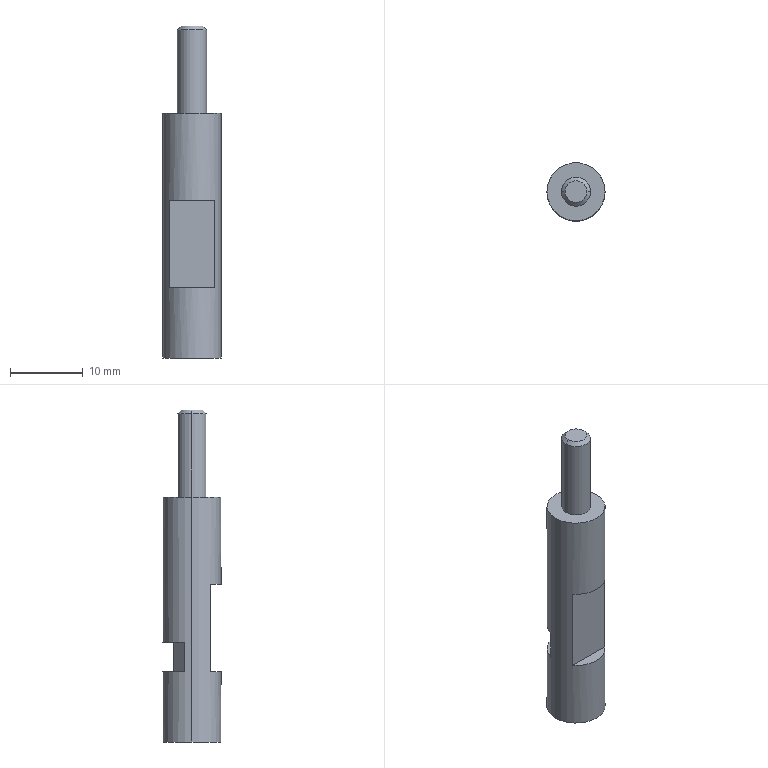Part | SolidWorks | features ICE 4, 3DProfileFeature 2, HoleWzd 2, Chamfer 1, Extrusion 1, RefAxis 1 | 1 solid | 24 faces | box 8 x 8 x 45.7 mm | volume 1609 mm3 | plane 11 | cylinder 8 | cone 5 | commonest cylinder face diameters 3.2 x4 4 x2 8 x2
STEP:
#1=CARTESIAN_POINT('',(-0.02022,1.6,10.1));
#2=VERTEX_POINT('',#1);
#3=CARTESIAN_POINT('',(-1.6,0.,11.446));
#4=VERTEX_POINT('',#3);
#5=CARTESIAN_POINT('',(-0.02022,1.6,10.1));
#6=CARTESIAN_POINT('',(-0.1403,1.598,10.1));
#7=CARTESIAN_POINT('',(-0.2616,1.583,10.114));
#8=CARTESIAN_POINT('',(-0.4907,1.527,10.166));
#9=CARTESIAN_POINT('',(-0.6,1.487,10.205));
#10=CARTESIAN_POINT('',(-0.8999,1.342,10.345));
#11=CARTESIAN_POINT('',(-1.065,1.21,10.473));
#12=CARTESIAN_POINT('',(-1.324,0.9196,10.753));
#13=CARTESIAN_POINT('',(-1.421,0.7579,10.908));
#14=CARTESIAN_POINT('',(-1.522,0.5024,11.141));
#15=CARTESIAN_POINT('',(-1.548,0.4151,11.219));
#16=CARTESIAN_POINT('',(-1.577,0.274,11.329));
#17=CARTESIAN_POINT('',(-1.585,0.225,11.365));
#18=CARTESIAN_POINT('',(-1.596,0.1195,11.423));
#19=CARTESIAN_POINT('',(-1.6,0.06134,11.446));
#20=CARTESIAN_POINT('',(-1.6,0.,11.446));
#21=B_SPLINE_CURVE_WITH_KNOTS('',3,(#5,#6,#7,#8,#9,#10,#11,#12,#13,#14,#15,#16,#17,#18,#19,#20),.UNSPECIFIED.,.F.,.F.,(4,2,2,2,2,2,2,4),(0.008715,0.009076,0.009436,0.01016,0.01088,0.01124,0.01142,0.0116),.UNSPECIFIED.);
#22=EDGE_CURVE('',#2,#4,#21,.T.);
#23=ORIENTED_EDGE('',*,*,#22,.F.);
#24=CARTESIAN_POINT('',(-0.02022,2.5,10.1));
#25=VERTEX_POINT('',#24);
#26=CARTESIAN_POINT('',(-0.02022,2.5,10.1));
#27=DIRECTION('',(0.,1.,0.));
#28=VECTOR('',#27,1000.);
#29=LINE('',#26,#28);
#30=EDGE_CURVE('',#2,#25,#29,.T.);
#31=ORIENTED_EDGE('',*,*,#30,.T.);
#32=CARTESIAN_POINT('',(-0.02022,2.5,13.3));
#33=VERTEX_POINT('',#32);
#34=CARTESIAN_POINT('',(-0.02022,2.5,11.7));
#35=DIRECTION('',(0.,1.,0.));
#36=DIRECTION('',(0.,0.,1.));
#37=AXIS2_PLACEMENT_3D('',#34,#35,#36);
#38=CIRCLE('',#37,1.6);
#39=EDGE_CURVE('',#25,#33,#38,.T.);
#40=ORIENTED_EDGE('',*,*,#39,.T.);
#41=CARTESIAN_POINT('',(-0.02022,1.6,13.3));
#42=VERTEX_POINT('',#41);
#43=CARTESIAN_POINT('',(-0.02022,2.5,13.3));
#44=DIRECTION('',(0.,1.,0.));
#45=VECTOR('',#44,1000.);
#46=LINE('',#43,#45);
#47=EDGE_CURVE('',#42,#33,#46,.T.);
#48=ORIENTED_EDGE('',*,*,#47,.F.);
#49=CARTESIAN_POINT('',(-1.6,0.,11.954));
#50=VERTEX_POINT('',#49);
#51=CARTESIAN_POINT('',(-1.6,0.,11.954));
#52=CARTESIAN_POINT('',(-1.6,0.06178,11.954));
#53=CARTESIAN_POINT('',(-1.596,0.1196,11.977));
#54=CARTESIAN_POINT('',(-1.585,0.2248,12.035));
#55=CARTESIAN_POINT('',(-1.577,0.2732,12.07));
#56=CARTESIAN_POINT('',(-1.548,0.4148,12.18));
#57=CARTESIAN_POINT('',(-1.522,0.5025,12.259));
#58=CARTESIAN_POINT('',(-1.455,0.6723,12.414));
#59=CARTESIAN_POINT('',(-1.414,0.7543,12.491));
#60=CARTESIAN_POINT('',(-1.317,0.9136,12.642));
#61=CARTESIAN_POINT('',(-1.26,0.9914,12.716));
#62=CARTESIAN_POINT('',(-1.13,1.137,12.857));
#63=CARTESIAN_POINT('',(-1.057,1.206,12.923));
#64=CARTESIAN_POINT('',(-0.8918,1.332,13.046));
#65=CARTESIAN_POINT('',(-0.7997,1.39,13.102));
#66=CARTESIAN_POINT('',(-0.6006,1.487,13.195));
#67=CARTESIAN_POINT('',(-0.4907,1.527,13.234));
#68=CARTESIAN_POINT('',(-0.2622,1.583,13.286));
#69=CARTESIAN_POINT('',(-0.1408,1.598,13.3));
#70=CARTESIAN_POINT('',(-0.02022,1.6,13.3));
#71=B_SPLINE_CURVE_WITH_KNOTS('',3,(#51,#52,#53,#54,#55,#56,#57,#58,#59,#60,#61,#62,#63,#64,#65,#66,#67,#68,#69,#70),.UNSPECIFIED.,.F.,.F.,(4,2,2,2,2,2,2,2,2,4),(0.,0.000181,0.000362,0.0007239,0.001086,0.001448,0.00181,0.002172,0.002534,0.002896),.UNSPECIFIED.);
#72=EDGE_CURVE('',#50,#42,#71,.T.);
#73=ORIENTED_EDGE('',*,*,#72,.F.);
#74=CARTESIAN_POINT('',(-0.02022,0.,11.7));
#75=DIRECTION('',(0.,1.,0.));
#76=DIRECTION('',(0.,0.,1.));
#77=AXIS2_PLACEMENT_3D('',#74,#75,#76);
#78=CIRCLE('',#77,1.6);
#79=EDGE_CURVE('',#4,#50,#78,.T.);
#80=ORIENTED_EDGE('',*,*,#79,.F.);
#81=EDGE_LOOP('',(#23,#31,#40,#48,#73,#80));
#82=FACE_OUTER_BOUND('',#81,.T.);
#83=CARTESIAN_POINT('',(-0.02022,2.5,11.7));
#84=DIRECTION('',(0.,1.,0.));
#85=DIRECTION('',(0.,0.,1.));
#86=AXIS2_PLACEMENT_3D('',#83,#84,#85);
#87=CYLINDRICAL_SURFACE('',#86,1.6);
#88=ADVANCED_FACE('',(#82),#87,.F.);
#89=CARTESIAN_POINT('',(1.6,0.,14.));
#90=VERTEX_POINT('',#89);
#91=CARTESIAN_POINT('',(-1.6,0.,14.));
#92=VERTEX_POINT('',#91);
#93=CARTESIAN_POINT('',(0.,0.,14.));
#94=DIRECTION('',(0.,0.,-1.));
#95=DIRECTION('',(-1.,0.,0.));
#96=AXIS2_PLACEMENT_3D('',#93,#94,#95);
#97=CIRCLE('',#96,1.6);
#98=EDGE_CURVE('',#90,#92,#97,.T.);
#99=ORIENTED_EDGE('',*,*,#98,.F.);
#100=CARTESIAN_POINT('',(1.6,0.,0.));
#101=VERTEX_POINT('',#100);
#102=CARTESIAN_POINT('',(1.6,0.,0.));
#103=DIRECTION('',(0.,0.,-1.));
#104=VECTOR('',#103,1000.);
#105=LINE('',#102,#104);
#106=EDGE_CURVE('',#90,#101,#105,.T.);
#107=ORIENTED_EDGE('',*,*,#106,.T.);
#108=CARTESIAN_POINT('',(-1.6,0.,0.));
#109=VERTEX_POINT('',#108);
#110=CARTESIAN_POINT('',(0.,0.,0.));
#111=DIRECTION('',(0.,0.,-1.));
#112=DIRECTION('',(-1.,0.,0.));
#113=AXIS2_PLACEMENT_3D('',#110,#111,#112);
#114=CIRCLE('',#113,1.6);
#115=EDGE_CURVE('',#101,#109,#114,.T.);
#116=ORIENTED_EDGE('',*,*,#115,.T.);
#117=CARTESIAN_POINT('',(-1.6,0.,0.));
#118=DIRECTION('',(0.,0.,-1.));
#119=VECTOR('',#118,1000.);
#120=LINE('',#117,#119);
#121=EDGE_CURVE('',#4,#109,#120,.T.);
#122=ORIENTED_EDGE('',*,*,#121,.F.);
#123=CARTESIAN_POINT('',(-1.6,0.,11.446));
#124=CARTESIAN_POINT('',(-1.6,-0.01594,11.614));
#125=CARTESIAN_POINT('',(-1.6,-0.01614,11.784));
#126=CARTESIAN_POINT('',(-1.6,0.,11.954));
#127=B_SPLINE_CURVE_WITH_KNOTS('',3,(#123,#124,#125,#126),.UNSPECIFIED.,.F.,.F.,(4,4),(0.0005362,0.001041),.UNSPECIFIED.);
#128=EDGE_CURVE('',#4,#50,#127,.T.);
#129=ORIENTED_EDGE('',*,*,#128,.T.);
#130=CARTESIAN_POINT('',(-1.6,0.,0.));
#131=DIRECTION('',(0.,0.,-1.));
#132=VECTOR('',#131,1000.);
#133=LINE('',#130,#132);
#134=EDGE_CURVE('',#92,#50,#133,.T.);
#135=ORIENTED_EDGE('',*,*,#134,.F.);
#136=EDGE_LOOP('',(#99,#107,#116,#122,#129,#135));
#137=FACE_OUTER_BOUND('',#136,.T.);
#138=CARTESIAN_POINT('',(0.,0.,0.));
#139=DIRECTION('',(0.,0.,-1.));
#140=DIRECTION('',(-1.,0.,0.));
#141=AXIS2_PLACEMENT_3D('',#138,#139,#140);
#142=CYLINDRICAL_SURFACE('',#141,1.6);
#143=ADVANCED_FACE('',(#137),#142,.F.);
#144=CARTESIAN_POINT('',(0.,0.,14.961));
#145=VERTEX_POINT('',#144);
#146=CARTESIAN_POINT('',(-1.6,0.,14.));
#147=DIRECTION('',(-0.8572,0.,-0.515));
#148=VECTOR('',#147,1000.);
#149=LINE('',#146,#148);
#150=EDGE_CURVE('',#145,#92,#149,.T.);
#151=ORIENTED_EDGE('',*,*,#150,.F.);
#152=CARTESIAN_POINT('',(1.6,0.,14.));
#153=DIRECTION('',(0.8572,0.,-0.515));
#154=VECTOR('',#153,1000.);
#155=LINE('',#152,#154);
#156=EDGE_CURVE('',#145,#90,#155,.T.);
#157=ORIENTED_EDGE('',*,*,#156,.T.);
#158=ORIENTED_EDGE('',*,*,#98,.T.);
#159=EDGE_LOOP('',(#151,#157,#158));
#160=FACE_OUTER_BOUND('',#159,.T.);
#161=CARTESIAN_POINT('',(0.,0.,14.));
#162=DIRECTION('',(0.,0.,-1.));
#163=DIRECTION('',(-1.,0.,0.));
#164=AXIS2_PLACEMENT_3D('',#161,#162,#163);
#165=CONICAL_SURFACE('',#164,1.6,1.03);
#166=ADVANCED_FACE('',(#160),#165,.F.);
#167=CARTESIAN_POINT('',(1.5,0.,45.7));
#168=VERTEX_POINT('',#167);
#169=CARTESIAN_POINT('',(-1.5,0.,45.7));
#170=VERTEX_POINT('',#169);
#171=CARTESIAN_POINT('',(0.,0.,45.7));
#172=DIRECTION('',(0.,0.,1.));
#173=DIRECTION('',(1.,0.,0.));
#174=AXIS2_PLACEMENT_3D('',#171,#172,#173);
#175=CIRCLE('',#174,1.5);
#176=EDGE_CURVE('',#168,#170,#175,.T.);
#177=ORIENTED_EDGE('',*,*,#176,.F.);
#178=CARTESIAN_POINT('',(2.,0.,45.2));
#179=VERTEX_POINT('',#178);
#180=CARTESIAN_POINT('',(1.5,0.,45.7));
#181=DIRECTION('',(0.7071,0.,-0.7071));
#182=VECTOR('',#181,1000.);
#183=LINE('',#180,#182);
#184=EDGE_CURVE('',#168,#179,#183,.T.);
#185=ORIENTED_EDGE('',*,*,#184,.T.);
#186=CARTESIAN_POINT('',(-2.,0.,45.2));
#187=VERTEX_POINT('',#186);
#188=CARTESIAN_POINT('',(0.,0.,45.2));
#189=DIRECTION('',(0.,0.,-1.));
#190=DIRECTION('',(1.,0.,0.));
#191=AXIS2_PLACEMENT_3D('',#188,#189,#190);
#192=CIRCLE('',#191,2.);
#193=EDGE_CURVE('',#187,#179,#192,.T.);
#194=ORIENTED_EDGE('',*,*,#193,.F.);
#195=CARTESIAN_POINT('',(-1.5,0.,45.7));
#196=DIRECTION('',(-0.7071,0.,-0.7071));
#197=VECTOR('',#196,1000.);
#198=LINE('',#195,#197);
#199=EDGE_CURVE('',#170,#187,#198,.T.);
#200=ORIENTED_EDGE('',*,*,#199,.F.);
#201=EDGE_LOOP('',(#177,#185,#194,#200));
#202=FACE_OUTER_BOUND('',#201,.T.);
#203=CARTESIAN_POINT('',(0.,0.,45.7));
#204=DIRECTION('',(0.,0.,-1.));
#205=DIRECTION('',(-1.,0.,0.));
#206=AXIS2_PLACEMENT_3D('',#203,#204,#205);
#207=CONICAL_SURFACE('',#206,1.5,0.7854);
#208=ADVANCED_FACE('',(#202),#207,.T.);
#209=ORIENTED_EDGE('',*,*,#193,.T.);
#210=CARTESIAN_POINT('',(2.,0.,33.7));
#211=VERTEX_POINT('',#210);
#212=CARTESIAN_POINT('',(2.,0.,45.7));
#213=DIRECTION('',(0.,0.,-1.));
#214=VECTOR('',#213,1000.);
#215=LINE('',#212,#214);
#216=EDGE_CURVE('',#179,#211,#215,.T.);
#217=ORIENTED_EDGE('',*,*,#216,.T.);
#218=CARTESIAN_POINT('',(-2.,0.,33.7));
#219=VERTEX_POINT('',#218);
#220=CARTESIAN_POINT('',(0.,0.,33.7));
#221=DIRECTION('',(0.,0.,1.));
#222=DIRECTION('',(1.,0.,0.));
#223=AXIS2_PLACEMENT_3D('',#220,#221,#222);
#224=CIRCLE('',#223,2.);
#225=EDGE_CURVE('',#211,#219,#224,.T.);
#226=ORIENTED_EDGE('',*,*,#225,.T.);
#227=CARTESIAN_POINT('',(-2.,0.,45.7));
#228=DIRECTION('',(0.,0.,-1.));
#229=VECTOR('',#228,1000.);
#230=LINE('',#227,#229);
#231=EDGE_CURVE('',#187,#219,#230,.T.);
#232=ORIENTED_EDGE('',*,*,#231,.F.);
#233=EDGE_LOOP('',(#209,#217,#226,#232));
#234=FACE_OUTER_BOUND('',#233,.T.);
#235=CARTESIAN_POINT('',(0.,0.,45.7));
#236=DIRECTION('',(0.,0.,-1.));
#237=DIRECTION('',(-1.,0.,0.));
#238=AXIS2_PLACEMENT_3D('',#235,#236,#237);
#239=CYLINDRICAL_SURFACE('',#238,2.);
#240=ADVANCED_FACE('',(#234),#239,.T.);
#241=CARTESIAN_POINT('',(3.708,1.5,9.7));
#242=VERTEX_POINT('',#241);
#243=CARTESIAN_POINT('',(-3.873,1.,9.7));
#244=VERTEX_POINT('',#243);
#245=CARTESIAN_POINT('',(0.,0.,9.7));
#246=DIRECTION('',(0.,0.,1.));
#247=DIRECTION('',(1.,0.,0.));
#248=AXIS2_PLACEMENT_3D('',#245,#246,#247);
#249=CIRCLE('',#248,4.);
#250=EDGE_CURVE('',#242,#244,#249,.T.);
#251=ORIENTED_EDGE('',*,*,#250,.F.);
#252=CARTESIAN_POINT('',(3.708,1.5,13.7));
#253=VERTEX_POINT('',#252);
#254=CARTESIAN_POINT('',(3.708,1.5,13.7));
#255=DIRECTION('',(0.,0.,-1.));
#256=VECTOR('',#255,1000.);
#257=LINE('',#254,#256);
#258=EDGE_CURVE('',#253,#242,#257,.T.);
#259=ORIENTED_EDGE('',*,*,#258,.F.);
#260=CARTESIAN_POINT('',(-3.873,1.,13.7));
#261=VERTEX_POINT('',#260);
#262=CARTESIAN_POINT('',(0.,0.,13.7));
#263=DIRECTION('',(0.,0.,1.));
#264=DIRECTION('',(1.,0.,0.));
#265=AXIS2_PLACEMENT_3D('',#262,#263,#264);
#266=CIRCLE('',#265,4.);
#267=EDGE_CURVE('',#253,#261,#266,.T.);
#268=ORIENTED_EDGE('',*,*,#267,.T.);
#269=CARTESIAN_POINT('',(-3.873,1.,13.7));
#270=DIRECTION('',(0.,0.,-1.));
#271=VECTOR('',#270,1000.);
#272=LINE('',#269,#271);
#273=EDGE_CURVE('',#261,#244,#272,.T.);
#274=ORIENTED_EDGE('',*,*,#273,.T.);
#275=EDGE_LOOP('',(#251,#259,#268,#274));
#276=FACE_BOUND('',#275,.T.);
#277=CARTESIAN_POINT('',(4.,0.,33.7));
#278=VERTEX_POINT('',#277);
#279=CARTESIAN_POINT('',(-4.,0.,33.7));
#280=VERTEX_POINT('',#279);
#281=CARTESIAN_POINT('',(0.,0.,33.7));
#282=DIRECTION('',(0.,0.,1.));
#283=DIRECTION('',(1.,0.,0.));
#284=AXIS2_PLACEMENT_3D('',#281,#282,#283);
#285=CIRCLE('',#284,4.);
#286=EDGE_CURVE('',#278,#280,#285,.T.);
#287=ORIENTED_EDGE('',*,*,#286,.F.);
#288=CARTESIAN_POINT('',(4.,0.,0.));
#289=VERTEX_POINT('',#288);
#290=CARTESIAN_POINT('',(4.,0.,9.7));
#291=DIRECTION('',(0.,0.,-1.));
#292=VECTOR('',#291,1000.);
#293=LINE('',#290,#292);
#294=EDGE_CURVE('',#278,#289,#293,.T.);
#295=ORIENTED_EDGE('',*,*,#294,.T.);
#296=CARTESIAN_POINT('',(-4.,0.,0.));
#297=VERTEX_POINT('',#296);
#298=CARTESIAN_POINT('',(0.,0.,0.));
#299=DIRECTION('',(0.,0.,1.));
#300=DIRECTION('',(1.,0.,0.));
#301=AXIS2_PLACEMENT_3D('',#298,#299,#300);
#302=CIRCLE('',#301,4.);
#303=EDGE_CURVE('',#289,#297,#302,.T.);
#304=ORIENTED_EDGE('',*,*,#303,.T.);
#305=CARTESIAN_POINT('',(-4.,0.,9.7));
#306=DIRECTION('',(0.,0.,-1.));
#307=VECTOR('',#306,1000.);
#308=LINE('',#305,#307);
#309=EDGE_CURVE('',#280,#297,#308,.T.);
#310=ORIENTED_EDGE('',*,*,#309,.F.);
#311=EDGE_LOOP('',(#287,#295,#304,#310));
#312=FACE_OUTER_BOUND('',#311,.T.);
#313=CARTESIAN_POINT('',(0.,0.,9.7));
#314=DIRECTION('',(0.,0.,-1.));
#315=DIRECTION('',(-1.,0.,0.));
#316=AXIS2_PLACEMENT_3D('',#313,#314,#315);
#317=CYLINDRICAL_SURFACE('',#316,4.);
#318=ADVANCED_FACE('',(#276,#312),#317,.T.);
#319=ORIENTED_EDGE('',*,*,#294,.F.);
#320=CARTESIAN_POINT('',(0.,0.,33.7));
#321=DIRECTION('',(0.,0.,1.));
#322=DIRECTION('',(1.,0.,0.));
#323=AXIS2_PLACEMENT_3D('',#320,#321,#322);
#324=CIRCLE('',#323,4.);
#325=EDGE_CURVE('',#280,#278,#324,.T.);
#326=ORIENTED_EDGE('',*,*,#325,.F.);
#327=ORIENTED_EDGE('',*,*,#309,.T.);
#328=CARTESIAN_POINT('',(0.,0.,0.));
#329=DIRECTION('',(0.,0.,1.));
#330=DIRECTION('',(1.,0.,0.));
#331=AXIS2_PLACEMENT_3D('',#328,#329,#330);
#332=CIRCLE('',#331,4.);
#333=EDGE_CURVE('',#297,#289,#332,.T.);
#334=ORIENTED_EDGE('',*,*,#333,.T.);
#335=EDGE_LOOP('',(#319,#326,#327,#334));
#336=FACE_OUTER_BOUND('',#335,.T.);
#337=CARTESIAN_POINT('',(-3.122,-2.5,21.7));
#338=VERTEX_POINT('',#337);
#339=CARTESIAN_POINT('',(-3.122,-2.5,9.7));
#340=VERTEX_POINT('',#339);
#341=CARTESIAN_POINT('',(-3.122,-2.5,13.7));
#342=DIRECTION('',(0.,0.,-1.));
#343=VECTOR('',#342,1000.);
#344=LINE('',#341,#343);
#345=EDGE_CURVE('',#338,#340,#344,.T.);
#346=ORIENTED_EDGE('',*,*,#345,.F.);
#347=CARTESIAN_POINT('',(3.122,-2.5,21.7));
#348=VERTEX_POINT('',#347);
#349=CARTESIAN_POINT('',(0.,0.,21.7));
#350=DIRECTION('',(0.,0.,1.));
#351=DIRECTION('',(1.,0.,0.));
#352=AXIS2_PLACEMENT_3D('',#349,#350,#351);
#353=CIRCLE('',#352,4.);
#354=EDGE_CURVE('',#338,#348,#353,.T.);
#355=ORIENTED_EDGE('',*,*,#354,.T.);
#356=CARTESIAN_POINT('',(3.122,-2.5,9.7));
#357=VERTEX_POINT('',#356);
#358=CARTESIAN_POINT('',(3.122,-2.5,13.7));
#359=DIRECTION('',(0.,0.,-1.));
#360=VECTOR('',#359,1000.);
#361=LINE('',#358,#360);
#362=EDGE_CURVE('',#348,#357,#361,.T.);
#363=ORIENTED_EDGE('',*,*,#362,.T.);
#364=CARTESIAN_POINT('',(0.,0.,9.7));
#365=DIRECTION('',(0.,0.,1.));
#366=DIRECTION('',(1.,0.,0.));
#367=AXIS2_PLACEMENT_3D('',#364,#365,#366);
#368=CIRCLE('',#367,4.);
#369=EDGE_CURVE('',#340,#357,#368,.T.);
#370=ORIENTED_EDGE('',*,*,#369,.F.);
#371=EDGE_LOOP('',(#346,#355,#363,#370));
#372=FACE_BOUND('',#371,.T.);
#373=CARTESIAN_POINT('',(0.,0.,9.7));
#374=DIRECTION('',(0.,0.,-1.));
#375=DIRECTION('',(-1.,0.,0.));
#376=AXIS2_PLACEMENT_3D('',#373,#374,#375);
#377=CYLINDRICAL_SURFACE('',#376,4.);
#378=ADVANCED_FACE('',(#336,#372),#377,.T.);
#379=CARTESIAN_POINT('',(-2.1,2.5,9.7));
#380=VERTEX_POINT('',#379);
#381=CARTESIAN_POINT('',(-3.873,1.,9.7));
#382=DIRECTION('',(-0.7634,-0.6459,0.));
#383=VECTOR('',#382,1000.);
#384=LINE('',#381,#383);
#385=EDGE_CURVE('',#380,#244,#384,.T.);
#386=ORIENTED_EDGE('',*,*,#385,.F.);
#387=CARTESIAN_POINT('',(2.1,2.5,9.7));
#388=VERTEX_POINT('',#387);
#389=CARTESIAN_POINT('',(-2.1,2.5,9.7));
#390=DIRECTION('',(-1.,0.,0.));
#391=VECTOR('',#390,1000.);
#392=LINE('',#389,#391);
#393=EDGE_CURVE('',#388,#380,#392,.T.);
#394=ORIENTED_EDGE('',*,*,#393,.F.);
#395=CARTESIAN_POINT('',(2.1,2.5,9.7));
#396=DIRECTION('',(-0.8492,0.5281,0.));
#397=VECTOR('',#396,1000.);
#398=LINE('',#395,#397);
#399=EDGE_CURVE('',#242,#388,#398,.T.);
#400=ORIENTED_EDGE('',*,*,#399,.F.);
#401=ORIENTED_EDGE('',*,*,#250,.T.);
#402=EDGE_LOOP('',(#386,#394,#400,#401));
#403=FACE_OUTER_BOUND('',#402,.T.);
#404=CARTESIAN_POINT('',(0.,0.,9.7));
#405=DIRECTION('',(0.,0.,1.));
#406=DIRECTION('',(1.,0.,0.));
#407=AXIS2_PLACEMENT_3D('',#404,#405,#406);
#408=PLANE('',#407);
#409=ADVANCED_FACE('',(#403),#408,.T.);
#410=CARTESIAN_POINT('',(-3.122,-2.5,9.7));
#411=DIRECTION('',(1.,0.,0.));
#412=VECTOR('',#411,1000.);
#413=LINE('',#410,#412);
#414=EDGE_CURVE('',#340,#357,#413,.T.);
#415=ORIENTED_EDGE('',*,*,#414,.F.);
#416=ORIENTED_EDGE('',*,*,#369,.T.);
#417=EDGE_LOOP('',(#415,#416));
#418=FACE_OUTER_BOUND('',#417,.T.);
#419=CARTESIAN_POINT('',(0.,0.,9.7));
#420=DIRECTION('',(0.,0.,1.));
#421=DIRECTION('',(1.,0.,0.));
#422=AXIS2_PLACEMENT_3D('',#419,#420,#421);
#423=PLANE('',#422);
#424=ADVANCED_FACE('',(#418),#423,.T.);
#425=CARTESIAN_POINT('',(0.,0.,0.));
#426=DIRECTION('',(0.,0.,-1.));
#427=DIRECTION('',(-1.,0.,0.));
#428=AXIS2_PLACEMENT_3D('',#425,#426,#427);
#429=CIRCLE('',#428,1.6);
#430=EDGE_CURVE('',#109,#101,#429,.T.);
#431=ORIENTED_EDGE('',*,*,#430,.F.);
#432=ORIENTED_EDGE('',*,*,#115,.F.);
#433=EDGE_LOOP('',(#431,#432));
#434=FACE_BOUND('',#433,.T.);
#435=ORIENTED_EDGE('',*,*,#333,.F.);
#436=ORIENTED_EDGE('',*,*,#303,.F.);
#437=EDGE_LOOP('',(#435,#436));
#438=FACE_OUTER_BOUND('',#437,.T.);
#439=CARTESIAN_POINT('',(0.,0.,0.));
#440=DIRECTION('',(0.,0.,1.));
#441=DIRECTION('',(1.,0.,0.));
#442=AXIS2_PLACEMENT_3D('',#439,#440,#441);
#443=PLANE('',#442);
#444=ADVANCED_FACE('',(#434,#438),#443,.F.);
#445=ORIENTED_EDGE('',*,*,#414,.T.);
#446=ORIENTED_EDGE('',*,*,#362,.F.);
#447=CARTESIAN_POINT('',(3.122,-2.5,21.7));
#448=DIRECTION('',(-1.,0.,0.));
#449=VECTOR('',#448,1000.);
#450=LINE('',#447,#449);
#451=EDGE_CURVE('',#348,#338,#450,.T.);
#452=ORIENTED_EDGE('',*,*,#451,.T.);
#453=ORIENTED_EDGE('',*,*,#345,.T.);
#454=EDGE_LOOP('',(#445,#446,#452,#453));
#455=FACE_OUTER_BOUND('',#454,.T.);
#456=CARTESIAN_POINT('',(-3.122,-2.5,13.7));
#457=DIRECTION('',(0.,1.,0.));
#458=DIRECTION('',(0.,0.,1.));
#459=AXIS2_PLACEMENT_3D('',#456,#457,#458);
#460=PLANE('',#459);
#461=ADVANCED_FACE('',(#455),#460,.F.);
#462=ORIENTED_EDGE('',*,*,#399,.T.);
#463=CARTESIAN_POINT('',(2.1,2.5,13.7));
#464=VERTEX_POINT('',#463);
#465=CARTESIAN_POINT('',(2.1,2.5,13.7));
#466=DIRECTION('',(0.,0.,-1.));
#467=VECTOR('',#466,1000.);
#468=LINE('',#465,#467);
#469=EDGE_CURVE('',#464,#388,#468,.T.);
#470=ORIENTED_EDGE('',*,*,#469,.F.);
#471=CARTESIAN_POINT('',(2.1,2.5,13.7));
#472=DIRECTION('',(-0.8492,0.5281,0.));
#473=VECTOR('',#472,1000.);
#474=LINE('',#471,#473);
#475=EDGE_CURVE('',#253,#464,#474,.T.);
#476=ORIENTED_EDGE('',*,*,#475,.F.);
#477=ORIENTED_EDGE('',*,*,#258,.T.);
#478=EDGE_LOOP('',(#462,#470,#476,#477));
#479=FACE_OUTER_BOUND('',#478,.T.);
#480=CARTESIAN_POINT('',(2.1,2.5,13.7));
#481=DIRECTION('',(-0.5281,-0.8492,0.));
#482=DIRECTION('',(0.8492,-0.5281,0.));
#483=AXIS2_PLACEMENT_3D('',#480,#481,#482);
#484=PLANE('',#483);
#485=ADVANCED_FACE('',(#479),#484,.F.);
#486=CARTESIAN_POINT('',(-0.02022,2.5,11.7));
#487=DIRECTION('',(0.,1.,0.));
#488=DIRECTION('',(0.,0.,1.));
#489=AXIS2_PLACEMENT_3D('',#486,#487,#488);
#490=CIRCLE('',#489,1.6);
#491=EDGE_CURVE('',#33,#25,#490,.T.);
#492=ORIENTED_EDGE('',*,*,#491,.F.);
#493=ORIENTED_EDGE('',*,*,#39,.F.);
#494=EDGE_LOOP('',(#492,#493));
#495=FACE_BOUND('',#494,.T.);
#496=ORIENTED_EDGE('',*,*,#393,.T.);
#497=CARTESIAN_POINT('',(-2.1,2.5,13.7));
#498=VERTEX_POINT('',#497);
#499=CARTESIAN_POINT('',(-2.1,2.5,13.7));
#500=DIRECTION('',(0.,0.,-1.));
#501=VECTOR('',#500,1000.);
#502=LINE('',#499,#501);
#503=EDGE_CURVE('',#498,#380,#502,.T.);
#504=ORIENTED_EDGE('',*,*,#503,.F.);
#505=CARTESIAN_POINT('',(-2.1,2.5,13.7));
#506=DIRECTION('',(-1.,0.,0.));
#507=VECTOR('',#506,1000.);
#508=LINE('',#505,#507);
#509=EDGE_CURVE('',#464,#498,#508,.T.);
#510=ORIENTED_EDGE('',*,*,#509,.F.);
#511=ORIENTED_EDGE('',*,*,#469,.T.);
#512=EDGE_LOOP('',(#496,#504,#510,#511));
#513=FACE_OUTER_BOUND('',#512,.T.);
#514=CARTESIAN_POINT('',(-2.1,2.5,13.7));
#515=DIRECTION('',(0.,-1.,0.));
#516=DIRECTION('',(0.,0.,-1.));
#517=AXIS2_PLACEMENT_3D('',#514,#515,#516);
#518=PLANE('',#517);
#519=ADVANCED_FACE('',(#495,#513),#518,.F.);
#520=ORIENTED_EDGE('',*,*,#385,.T.);
#521=ORIENTED_EDGE('',*,*,#273,.F.);
#522=CARTESIAN_POINT('',(-3.873,1.,13.7));
#523=DIRECTION('',(-0.7634,-0.6459,0.));
#524=VECTOR('',#523,1000.);
#525=LINE('',#522,#524);
#526=EDGE_CURVE('',#498,#261,#525,.T.);
#527=ORIENTED_EDGE('',*,*,#526,.F.);
#528=ORIENTED_EDGE('',*,*,#503,.T.);
#529=EDGE_LOOP('',(#520,#521,#527,#528));
#530=FACE_OUTER_BOUND('',#529,.T.);
#531=CARTESIAN_POINT('',(-3.873,1.,13.7));
#532=DIRECTION('',(0.6459,-0.7634,0.));
#533=DIRECTION('',(0.7634,0.6459,0.));
#534=AXIS2_PLACEMENT_3D('',#531,#532,#533);
#535=PLANE('',#534);
#536=ADVANCED_FACE('',(#530),#535,.F.);
#537=ORIENTED_EDGE('',*,*,#267,.F.);
#538=ORIENTED_EDGE('',*,*,#475,.T.);
#539=ORIENTED_EDGE('',*,*,#509,.T.);
#540=ORIENTED_EDGE('',*,*,#526,.T.);
#541=EDGE_LOOP('',(#537,#538,#539,#540));
#542=FACE_OUTER_BOUND('',#541,.T.);
#543=CARTESIAN_POINT('',(0.,0.,13.7));
#544=DIRECTION('',(0.,0.,1.));
#545=DIRECTION('',(1.,0.,0.));
#546=AXIS2_PLACEMENT_3D('',#543,#544,#545);
#547=PLANE('',#546);
#548=ADVANCED_FACE('',(#542),#547,.F.);
#549=CARTESIAN_POINT('',(0.,0.,33.7));
#550=DIRECTION('',(0.,0.,1.));
#551=DIRECTION('',(1.,0.,0.));
#552=AXIS2_PLACEMENT_3D('',#549,#550,#551);
#553=CIRCLE('',#552,2.);
#554=EDGE_CURVE('',#219,#211,#553,.T.);
#555=ORIENTED_EDGE('',*,*,#554,.F.);
#556=ORIENTED_EDGE('',*,*,#225,.F.);
#557=EDGE_LOOP('',(#555,#556));
#558=FACE_BOUND('',#557,.T.);
#559=ORIENTED_EDGE('',*,*,#325,.T.);
#560=ORIENTED_EDGE('',*,*,#286,.T.);
#561=EDGE_LOOP('',(#559,#560));
#562=FACE_OUTER_BOUND('',#561,.T.);
#563=CARTESIAN_POINT('',(0.,0.,33.7));
#564=DIRECTION('',(0.,0.,1.));
#565=DIRECTION('',(1.,0.,0.));
#566=AXIS2_PLACEMENT_3D('',#563,#564,#565);
#567=PLANE('',#566);
#568=ADVANCED_FACE('',(#558,#562),#567,.T.);
#569=ORIENTED_EDGE('',*,*,#216,.F.);
#570=CARTESIAN_POINT('',(0.,0.,45.2));
#571=DIRECTION('',(0.,0.,-1.));
#572=DIRECTION('',(1.,0.,0.));
#573=AXIS2_PLACEMENT_3D('',#570,#571,#572);
#574=CIRCLE('',#573,2.);
#575=EDGE_CURVE('',#179,#187,#574,.T.);
#576=ORIENTED_EDGE('',*,*,#575,.T.);
#577=ORIENTED_EDGE('',*,*,#231,.T.);
#578=ORIENTED_EDGE('',*,*,#554,.T.);
#579=EDGE_LOOP('',(#569,#576,#577,#578));
#580=FACE_OUTER_BOUND('',#579,.T.);
#581=CARTESIAN_POINT('',(0.,0.,45.7));
#582=DIRECTION('',(0.,0.,-1.));
#583=DIRECTION('',(-1.,0.,0.));
#584=AXIS2_PLACEMENT_3D('',#581,#582,#583);
#585=CYLINDRICAL_SURFACE('',#584,2.);
#586=ADVANCED_FACE('',(#580),#585,.T.);
#587=CARTESIAN_POINT('',(0.,0.,45.7));
#588=DIRECTION('',(0.,0.,1.));
#589=DIRECTION('',(1.,0.,0.));
#590=AXIS2_PLACEMENT_3D('',#587,#588,#589);
#591=CIRCLE('',#590,1.5);
#592=EDGE_CURVE('',#170,#168,#591,.T.);
#593=ORIENTED_EDGE('',*,*,#592,.T.);
#594=ORIENTED_EDGE('',*,*,#176,.T.);
#595=EDGE_LOOP('',(#593,#594));
#596=FACE_OUTER_BOUND('',#595,.T.);
#597=CARTESIAN_POINT('',(0.,0.,45.7));
#598=DIRECTION('',(0.,0.,1.));
#599=DIRECTION('',(1.,0.,0.));
#600=AXIS2_PLACEMENT_3D('',#597,#598,#599);
#601=PLANE('',#600);
#602=ADVANCED_FACE('',(#596),#601,.T.);
#603=ORIENTED_EDGE('',*,*,#184,.F.);
#604=ORIENTED_EDGE('',*,*,#592,.F.);
#605=ORIENTED_EDGE('',*,*,#199,.T.);
#606=ORIENTED_EDGE('',*,*,#575,.F.);
#607=EDGE_LOOP('',(#603,#604,#605,#606));
#608=FACE_OUTER_BOUND('',#607,.T.);
#609=CARTESIAN_POINT('',(0.,0.,45.7));
#610=DIRECTION('',(0.,0.,-1.));
#611=DIRECTION('',(-1.,0.,0.));
#612=AXIS2_PLACEMENT_3D('',#609,#610,#611);
#613=CONICAL_SURFACE('',#612,1.5,0.7854);
#614=ADVANCED_FACE('',(#608),#613,.T.);
#615=ORIENTED_EDGE('',*,*,#354,.F.);
#616=ORIENTED_EDGE('',*,*,#451,.F.);
#617=EDGE_LOOP('',(#615,#616));
#618=FACE_OUTER_BOUND('',#617,.T.);
#619=CARTESIAN_POINT('',(0.,0.,21.7));
#620=DIRECTION('',(0.,0.,1.));
#621=DIRECTION('',(1.,0.,0.));
#622=AXIS2_PLACEMENT_3D('',#619,#620,#621);
#623=PLANE('',#622);
#624=ADVANCED_FACE('',(#618),#623,.F.);
#625=ORIENTED_EDGE('',*,*,#156,.F.);
#626=ORIENTED_EDGE('',*,*,#150,.T.);
#627=CARTESIAN_POINT('',(0.,0.,14.));
#628=DIRECTION('',(0.,0.,-1.));
#629=DIRECTION('',(-1.,0.,0.));
#630=AXIS2_PLACEMENT_3D('',#627,#628,#629);
#631=CIRCLE('',#630,1.6);
#632=EDGE_CURVE('',#92,#90,#631,.T.);
#633=ORIENTED_EDGE('',*,*,#632,.T.);
#634=EDGE_LOOP('',(#625,#626,#633));
#635=FACE_OUTER_BOUND('',#634,.T.);
#636=CARTESIAN_POINT('',(0.,0.,14.));
#637=DIRECTION('',(0.,0.,-1.));
#638=DIRECTION('',(-1.,0.,0.));
#639=AXIS2_PLACEMENT_3D('',#636,#637,#638);
#640=CONICAL_SURFACE('',#639,1.6,1.03);
#641=ADVANCED_FACE('',(#635),#640,.F.);
#642=ORIENTED_EDGE('',*,*,#106,.F.);
#643=ORIENTED_EDGE('',*,*,#632,.F.);
#644=ORIENTED_EDGE('',*,*,#134,.T.);
#645=ORIENTED_EDGE('',*,*,#72,.T.);
#646=CARTESIAN_POINT('',(-0.02022,1.6,13.3));
#647=CARTESIAN_POINT('',(0.1009,1.601,13.3));
#648=CARTESIAN_POINT('',(0.2223,1.589,13.286));
#649=CARTESIAN_POINT('',(0.4545,1.539,13.233));
#650=CARTESIAN_POINT('',(0.5643,1.501,13.194));
#651=CARTESIAN_POINT('',(0.7677,1.408,13.097));
#652=CARTESIAN_POINT('',(0.8593,1.354,13.041));
#653=CARTESIAN_POINT('',(1.026,1.232,12.915));
#654=CARTESIAN_POINT('',(1.102,1.164,12.845));
#655=CARTESIAN_POINT('',(1.299,0.954,12.627));
#656=CARTESIAN_POINT('',(1.397,0.798,12.465));
#657=CARTESIAN_POINT('',(1.5,0.5639,12.208));
#658=CARTESIAN_POINT('',(1.526,0.4854,12.121));
#659=CARTESIAN_POINT('',(1.556,0.3751,11.98));
#660=CARTESIAN_POINT('',(1.564,0.3392,11.931));
#661=CARTESIAN_POINT('',(1.576,0.2788,11.825));
#662=CARTESIAN_POINT('',(1.58,0.2547,11.766));
#663=CARTESIAN_POINT('',(1.58,0.2525,11.643));
#664=CARTESIAN_POINT('',(1.576,0.2754,11.583));
#665=CARTESIAN_POINT('',(1.565,0.3339,11.477));
#666=CARTESIAN_POINT('',(1.557,0.3695,11.428));
#667=CARTESIAN_POINT('',(1.528,0.4805,11.285));
#668=CARTESIAN_POINT('',(1.501,0.5594,11.197));
#669=CARTESIAN_POINT('',(1.4,0.7935,10.94));
#670=CARTESIAN_POINT('',(1.301,0.9506,10.777));
#671=CARTESIAN_POINT('',(1.038,1.232,10.484));
#672=CARTESIAN_POINT('',(0.8705,1.361,10.352));
#673=CARTESIAN_POINT('',(0.5669,1.5,10.207));
#674=CARTESIAN_POINT('',(0.4555,1.538,10.168));
#675=CARTESIAN_POINT('',(0.2242,1.589,10.114));
#676=CARTESIAN_POINT('',(0.101,1.601,10.1));
#677=CARTESIAN_POINT('',(-0.02022,1.6,10.1));
#678=B_SPLINE_CURVE_WITH_KNOTS('',3,(#646,#647,#648,#649,#650,#651,#652,#653,#654,#655,#656,#657,#658,#659,#660,#661,#662,#663,#664,#665,#666,#667,#668,#669,#670,#671,#672,#673,#674,#675,#676,#677),.UNSPECIFIED.,.F.,.F.,(4,2,2,2,2,2,2,2,2,2,2,2,2,2,2,4),(0.002896,0.003259,0.003623,0.003987,0.004351,0.005078,0.005442,0.005624,0.005805,0.005987,0.006169,0.006533,0.00726,0.007988,0.008351,0.008715),.UNSPECIFIED.);
#679=EDGE_CURVE('',#42,#2,#678,.T.);
#680=ORIENTED_EDGE('',*,*,#679,.T.);
#681=ORIENTED_EDGE('',*,*,#22,.T.);
#682=ORIENTED_EDGE('',*,*,#121,.T.);
#683=ORIENTED_EDGE('',*,*,#430,.T.);
#684=EDGE_LOOP('',(#642,#643,#644,#645,#680,#681,#682,#683));
#685=FACE_OUTER_BOUND('',#684,.T.);
#686=CARTESIAN_POINT('',(0.,0.,0.));
#687=DIRECTION('',(0.,0.,-1.));
#688=DIRECTION('',(-1.,0.,0.));
#689=AXIS2_PLACEMENT_3D('',#686,#687,#688);
#690=CYLINDRICAL_SURFACE('',#689,1.6);
#691=ADVANCED_FACE('',(#685),#690,.F.);
#692=ORIENTED_EDGE('',*,*,#79,.T.);
#693=ORIENTED_EDGE('',*,*,#128,.F.);
#694=EDGE_LOOP('',(#692,#693));
#695=FACE_OUTER_BOUND('',#694,.T.);
#696=CARTESIAN_POINT('',(-0.02022,0.,11.7));
#697=DIRECTION('',(0.,1.,0.));
#698=DIRECTION('',(0.,0.,1.));
#699=AXIS2_PLACEMENT_3D('',#696,#697,#698);
#700=CONICAL_SURFACE('',#699,1.6,1.03);
#701=ADVANCED_FACE('',(#695),#700,.F.);
#702=ORIENTED_EDGE('',*,*,#30,.F.);
#703=ORIENTED_EDGE('',*,*,#679,.F.);
#704=ORIENTED_EDGE('',*,*,#47,.T.);
#705=ORIENTED_EDGE('',*,*,#491,.T.);
#706=EDGE_LOOP('',(#702,#703,#704,#705));
#707=FACE_OUTER_BOUND('',#706,.T.);
#708=CARTESIAN_POINT('',(-0.02022,2.5,11.7));
#709=DIRECTION('',(0.,1.,0.));
#710=DIRECTION('',(0.,0.,1.));
#711=AXIS2_PLACEMENT_3D('',#708,#709,#710);
#712=CYLINDRICAL_SURFACE('',#711,1.6);
#713=ADVANCED_FACE('',(#707),#712,.F.);
#714=CLOSED_SHELL('',(#88,#143,#166,#208,#240,#318,#378,#409,#424,#444,#461,#485,#519,#536,#548,#568,#586,#602,#614,#624,#641,#691,#701,#713));
#715=MANIFOLD_SOLID_BREP('',#714);
#716=CARTESIAN_POINT('',(0.,0.,0.));
#717=DIRECTION('',(0.,0.,1.));
#718=DIRECTION('',(1.,0.,0.));
#719=AXIS2_PLACEMENT_3D('',#716,#717,#718);
#720=(LENGTH_UNIT()NAMED_UNIT(*)SI_UNIT(.MILLI.,.METRE.));
#721=UNCERTAINTY_MEASURE_WITH_UNIT(LENGTH_MEASURE(0.00001),#720,'','');
#722=(NAMED_UNIT(*)PLANE_ANGLE_UNIT()SI_UNIT($,.RADIAN.));
#723=(NAMED_UNIT(*)SI_UNIT($,.STERADIAN.)SOLID_ANGLE_UNIT());
#724=(GEOMETRIC_REPRESENTATION_CONTEXT(3)GLOBAL_UNCERTAINTY_ASSIGNED_CONTEXT((#721))GLOBAL_UNIT_ASSIGNED_CONTEXT((#720,#722,#723))REPRESENTATION_CONTEXT('',''));
#725=ADVANCED_BREP_SHAPE_REPRESENTATION('',(#715,#719),#724);